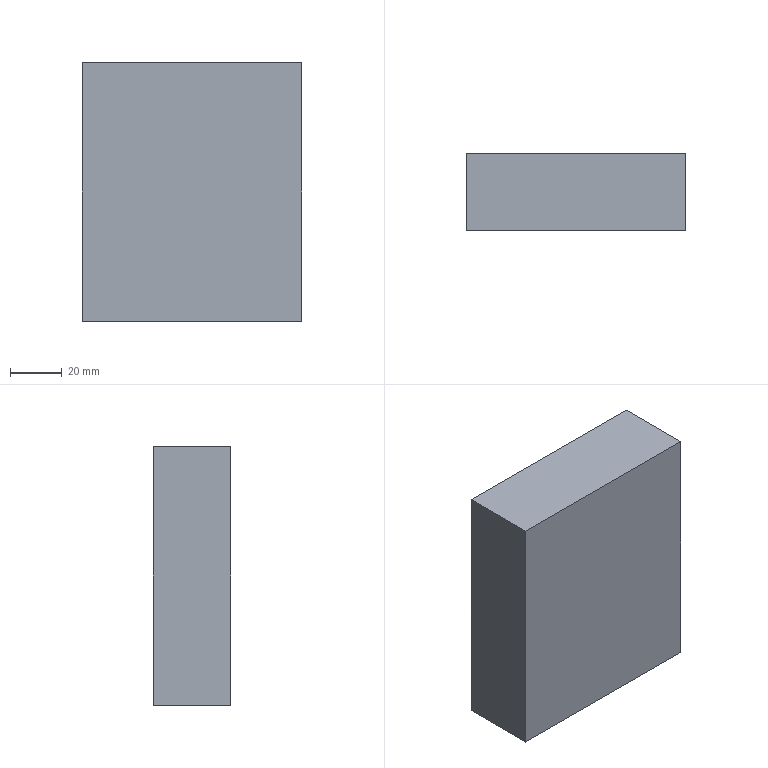Part | SolidWorks | features Extrusion 1 | 1 solid | 6 faces | box 85 x 30 x 100 mm | volume 255000 mm3 | plane 6
STEP:
#1=CARTESIAN_POINT('',(0.,30.,0.));
#2=VERTEX_POINT('',#1);
#3=CARTESIAN_POINT('',(0.,0.,0.));
#4=VERTEX_POINT('',#3);
#5=CARTESIAN_POINT('',(0.,0.,0.));
#6=DIRECTION('',(0.,-1.,0.));
#7=VECTOR('',#6,1000.);
#8=LINE('',#5,#7);
#9=EDGE_CURVE('',#2,#4,#8,.T.);
#10=ORIENTED_EDGE('',*,*,#9,.T.);
#11=CARTESIAN_POINT('',(85.,0.,0.));
#12=VERTEX_POINT('',#11);
#13=CARTESIAN_POINT('',(85.,0.,0.));
#14=DIRECTION('',(-1.,0.,0.));
#15=VECTOR('',#14,1000.);
#16=LINE('',#13,#15);
#17=EDGE_CURVE('',#12,#4,#16,.T.);
#18=ORIENTED_EDGE('',*,*,#17,.F.);
#19=CARTESIAN_POINT('',(85.,30.,0.));
#20=VERTEX_POINT('',#19);
#21=CARTESIAN_POINT('',(85.,0.,0.));
#22=DIRECTION('',(0.,-1.,0.));
#23=VECTOR('',#22,1000.);
#24=LINE('',#21,#23);
#25=EDGE_CURVE('',#20,#12,#24,.T.);
#26=ORIENTED_EDGE('',*,*,#25,.F.);
#27=CARTESIAN_POINT('',(85.,30.,0.));
#28=DIRECTION('',(-1.,0.,0.));
#29=VECTOR('',#28,1000.);
#30=LINE('',#27,#29);
#31=EDGE_CURVE('',#20,#2,#30,.T.);
#32=ORIENTED_EDGE('',*,*,#31,.T.);
#33=EDGE_LOOP('',(#10,#18,#26,#32));
#34=FACE_OUTER_BOUND('',#33,.T.);
#35=CARTESIAN_POINT('',(85.,0.,0.));
#36=DIRECTION('',(0.,0.,-1.));
#37=DIRECTION('',(-1.,0.,0.));
#38=AXIS2_PLACEMENT_3D('',#35,#36,#37);
#39=PLANE('',#38);
#40=ADVANCED_FACE('',(#34),#39,.F.);
#41=CARTESIAN_POINT('',(0.,0.,-100.));
#42=VERTEX_POINT('',#41);
#43=CARTESIAN_POINT('',(0.,0.,0.));
#44=DIRECTION('',(0.,0.,-1.));
#45=VECTOR('',#44,1000.);
#46=LINE('',#43,#45);
#47=EDGE_CURVE('',#4,#42,#46,.T.);
#48=ORIENTED_EDGE('',*,*,#47,.T.);
#49=CARTESIAN_POINT('',(85.,0.,-100.));
#50=VERTEX_POINT('',#49);
#51=CARTESIAN_POINT('',(85.,0.,-100.));
#52=DIRECTION('',(-1.,0.,0.));
#53=VECTOR('',#52,1000.);
#54=LINE('',#51,#53);
#55=EDGE_CURVE('',#50,#42,#54,.T.);
#56=ORIENTED_EDGE('',*,*,#55,.F.);
#57=CARTESIAN_POINT('',(85.,0.,0.));
#58=DIRECTION('',(0.,0.,-1.));
#59=VECTOR('',#58,1000.);
#60=LINE('',#57,#59);
#61=EDGE_CURVE('',#12,#50,#60,.T.);
#62=ORIENTED_EDGE('',*,*,#61,.F.);
#63=ORIENTED_EDGE('',*,*,#17,.T.);
#64=EDGE_LOOP('',(#48,#56,#62,#63));
#65=FACE_OUTER_BOUND('',#64,.T.);
#66=CARTESIAN_POINT('',(85.,0.,0.));
#67=DIRECTION('',(0.,1.,0.));
#68=DIRECTION('',(0.,0.,1.));
#69=AXIS2_PLACEMENT_3D('',#66,#67,#68);
#70=PLANE('',#69);
#71=ADVANCED_FACE('',(#65),#70,.F.);
#72=CARTESIAN_POINT('',(0.,30.,-100.));
#73=VERTEX_POINT('',#72);
#74=CARTESIAN_POINT('',(0.,0.,-100.));
#75=DIRECTION('',(0.,1.,0.));
#76=VECTOR('',#75,1000.);
#77=LINE('',#74,#76);
#78=EDGE_CURVE('',#42,#73,#77,.T.);
#79=ORIENTED_EDGE('',*,*,#78,.T.);
#80=CARTESIAN_POINT('',(85.,30.,-100.));
#81=VERTEX_POINT('',#80);
#82=CARTESIAN_POINT('',(85.,30.,-100.));
#83=DIRECTION('',(-1.,0.,0.));
#84=VECTOR('',#83,1000.);
#85=LINE('',#82,#84);
#86=EDGE_CURVE('',#81,#73,#85,.T.);
#87=ORIENTED_EDGE('',*,*,#86,.F.);
#88=CARTESIAN_POINT('',(85.,0.,-100.));
#89=DIRECTION('',(0.,1.,0.));
#90=VECTOR('',#89,1000.);
#91=LINE('',#88,#90);
#92=EDGE_CURVE('',#50,#81,#91,.T.);
#93=ORIENTED_EDGE('',*,*,#92,.F.);
#94=ORIENTED_EDGE('',*,*,#55,.T.);
#95=EDGE_LOOP('',(#79,#87,#93,#94));
#96=FACE_OUTER_BOUND('',#95,.T.);
#97=CARTESIAN_POINT('',(85.,0.,-100.));
#98=DIRECTION('',(0.,0.,1.));
#99=DIRECTION('',(1.,0.,0.));
#100=AXIS2_PLACEMENT_3D('',#97,#98,#99);
#101=PLANE('',#100);
#102=ADVANCED_FACE('',(#96),#101,.F.);
#103=CARTESIAN_POINT('',(0.,30.,0.));
#104=DIRECTION('',(0.,0.,1.));
#105=VECTOR('',#104,1000.);
#106=LINE('',#103,#105);
#107=EDGE_CURVE('',#73,#2,#106,.T.);
#108=ORIENTED_EDGE('',*,*,#107,.T.);
#109=ORIENTED_EDGE('',*,*,#31,.F.);
#110=CARTESIAN_POINT('',(85.,30.,0.));
#111=DIRECTION('',(0.,0.,1.));
#112=VECTOR('',#111,1000.);
#113=LINE('',#110,#112);
#114=EDGE_CURVE('',#81,#20,#113,.T.);
#115=ORIENTED_EDGE('',*,*,#114,.F.);
#116=ORIENTED_EDGE('',*,*,#86,.T.);
#117=EDGE_LOOP('',(#108,#109,#115,#116));
#118=FACE_OUTER_BOUND('',#117,.T.);
#119=CARTESIAN_POINT('',(85.,30.,0.));
#120=DIRECTION('',(0.,-1.,0.));
#121=DIRECTION('',(0.,0.,-1.));
#122=AXIS2_PLACEMENT_3D('',#119,#120,#121);
#123=PLANE('',#122);
#124=ADVANCED_FACE('',(#118),#123,.F.);
#125=ORIENTED_EDGE('',*,*,#25,.T.);
#126=ORIENTED_EDGE('',*,*,#61,.T.);
#127=ORIENTED_EDGE('',*,*,#92,.T.);
#128=ORIENTED_EDGE('',*,*,#114,.T.);
#129=EDGE_LOOP('',(#125,#126,#127,#128));
#130=FACE_OUTER_BOUND('',#129,.T.);
#131=CARTESIAN_POINT('',(85.,0.,0.));
#132=DIRECTION('',(-1.,0.,0.));
#133=DIRECTION('',(0.,0.,1.));
#134=AXIS2_PLACEMENT_3D('',#131,#132,#133);
#135=PLANE('',#134);
#136=ADVANCED_FACE('',(#130),#135,.F.);
#137=ORIENTED_EDGE('',*,*,#9,.F.);
#138=ORIENTED_EDGE('',*,*,#107,.F.);
#139=ORIENTED_EDGE('',*,*,#78,.F.);
#140=ORIENTED_EDGE('',*,*,#47,.F.);
#141=EDGE_LOOP('',(#137,#138,#139,#140));
#142=FACE_OUTER_BOUND('',#141,.T.);
#143=CARTESIAN_POINT('',(0.,0.,0.));
#144=DIRECTION('',(-1.,0.,0.));
#145=DIRECTION('',(0.,0.,1.));
#146=AXIS2_PLACEMENT_3D('',#143,#144,#145);
#147=PLANE('',#146);
#148=ADVANCED_FACE('',(#142),#147,.T.);
#149=CLOSED_SHELL('',(#40,#71,#102,#124,#136,#148));
#150=MANIFOLD_SOLID_BREP('',#149);
#151=CARTESIAN_POINT('',(0.,0.,0.));
#152=DIRECTION('',(0.,0.,1.));
#153=DIRECTION('',(1.,0.,0.));
#154=AXIS2_PLACEMENT_3D('',#151,#152,#153);
#155=(LENGTH_UNIT()NAMED_UNIT(*)SI_UNIT(.MILLI.,.METRE.));
#156=UNCERTAINTY_MEASURE_WITH_UNIT(LENGTH_MEASURE(0.00001),#155,'','');
#157=(NAMED_UNIT(*)PLANE_ANGLE_UNIT()SI_UNIT($,.RADIAN.));
#158=(NAMED_UNIT(*)SI_UNIT($,.STERADIAN.)SOLID_ANGLE_UNIT());
#159=(GEOMETRIC_REPRESENTATION_CONTEXT(3)GLOBAL_UNCERTAINTY_ASSIGNED_CONTEXT((#156))GLOBAL_UNIT_ASSIGNED_CONTEXT((#155,#157,#158))REPRESENTATION_CONTEXT('',''));
#160=ADVANCED_BREP_SHAPE_REPRESENTATION('',(#150,#154),#159);